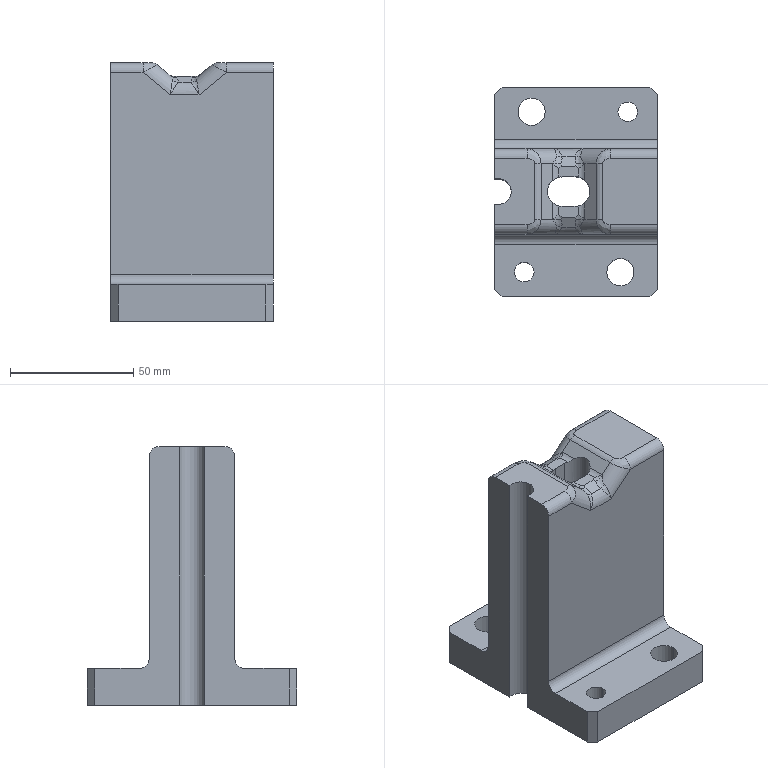Part | STEP file | 1_id58_x_t | 1 solid | 84 faces | box 66 x 85 x 105 mm | volume 245163 mm3 | cylinder 35 | plane 33 | spline 16 | commonest cylinder face diameters 8 x12 12 x8 6 x4 7.938 x4 11 x4 10.524 x2